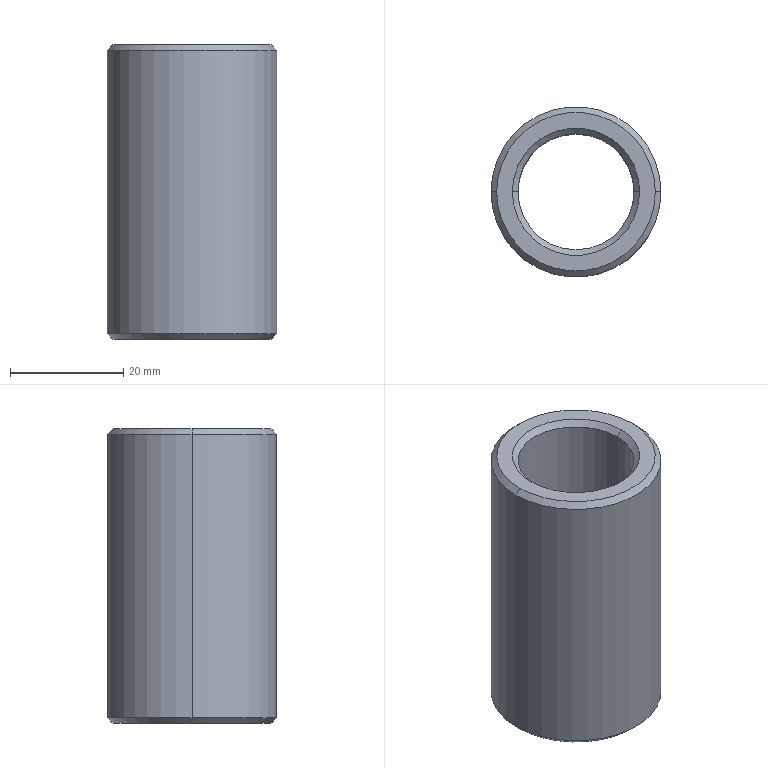Part | SolidWorks | features Chamfer 1, Extrusion 1 | 1 solid | 14 faces | box 30 x 30 x 52 mm | volume 19435 mm3 | cone 8 | cylinder 4 | plane 2 | commonest cylinder face diameters 20.5 x2 30 x2
STEP:
#1=CARTESIAN_POINT('',(-10.25,0.,25.));
#2=VERTEX_POINT('',#1);
#3=CARTESIAN_POINT('',(10.25,0.,25.));
#4=VERTEX_POINT('',#3);
#5=CARTESIAN_POINT('',(0.,0.,25.));
#6=DIRECTION('',(0.,0.,1.));
#7=DIRECTION('',(1.,0.,0.));
#8=AXIS2_PLACEMENT_3D('',#5,#6,#7);
#9=CIRCLE('',#8,10.25);
#10=EDGE_CURVE('',#2,#4,#9,.T.);
#11=ORIENTED_EDGE('',*,*,#10,.F.);
#12=CARTESIAN_POINT('',(-11.25,0.,26.));
#13=VERTEX_POINT('',#12);
#14=CARTESIAN_POINT('',(-10.25,0.,25.));
#15=DIRECTION('',(-0.7071,0.,0.7071));
#16=VECTOR('',#15,1000.);
#17=LINE('',#14,#16);
#18=EDGE_CURVE('',#2,#13,#17,.T.);
#19=ORIENTED_EDGE('',*,*,#18,.T.);
#20=CARTESIAN_POINT('',(11.25,0.,26.));
#21=VERTEX_POINT('',#20);
#22=CARTESIAN_POINT('',(0.,0.,26.));
#23=DIRECTION('',(0.,0.,-1.));
#24=DIRECTION('',(1.,0.,0.));
#25=AXIS2_PLACEMENT_3D('',#22,#23,#24);
#26=CIRCLE('',#25,11.25);
#27=EDGE_CURVE('',#21,#13,#26,.T.);
#28=ORIENTED_EDGE('',*,*,#27,.F.);
#29=CARTESIAN_POINT('',(10.25,0.,25.));
#30=DIRECTION('',(0.7071,0.,0.7071));
#31=VECTOR('',#30,1000.);
#32=LINE('',#29,#31);
#33=EDGE_CURVE('',#4,#21,#32,.T.);
#34=ORIENTED_EDGE('',*,*,#33,.F.);
#35=EDGE_LOOP('',(#11,#19,#28,#34));
#36=FACE_OUTER_BOUND('',#35,.T.);
#37=CARTESIAN_POINT('',(0.,0.,25.));
#38=DIRECTION('',(0.,0.,1.));
#39=DIRECTION('',(1.,0.,0.));
#40=AXIS2_PLACEMENT_3D('',#37,#38,#39);
#41=CONICAL_SURFACE('',#40,10.25,0.7854);
#42=ADVANCED_FACE('',(#36),#41,.F.);
#43=CARTESIAN_POINT('',(14.,0.,26.));
#44=VERTEX_POINT('',#43);
#45=CARTESIAN_POINT('',(-14.,0.,26.));
#46=VERTEX_POINT('',#45);
#47=CARTESIAN_POINT('',(0.,0.,26.));
#48=DIRECTION('',(0.,0.,1.));
#49=DIRECTION('',(1.,0.,0.));
#50=AXIS2_PLACEMENT_3D('',#47,#48,#49);
#51=CIRCLE('',#50,14.);
#52=EDGE_CURVE('',#44,#46,#51,.T.);
#53=ORIENTED_EDGE('',*,*,#52,.F.);
#54=CARTESIAN_POINT('',(15.,0.,25.));
#55=VERTEX_POINT('',#54);
#56=CARTESIAN_POINT('',(14.,0.,26.));
#57=DIRECTION('',(0.7071,0.,-0.7071));
#58=VECTOR('',#57,1000.);
#59=LINE('',#56,#58);
#60=EDGE_CURVE('',#44,#55,#59,.T.);
#61=ORIENTED_EDGE('',*,*,#60,.T.);
#62=CARTESIAN_POINT('',(-15.,0.,25.));
#63=VERTEX_POINT('',#62);
#64=CARTESIAN_POINT('',(0.,0.,25.));
#65=DIRECTION('',(0.,0.,-1.));
#66=DIRECTION('',(1.,0.,0.));
#67=AXIS2_PLACEMENT_3D('',#64,#65,#66);
#68=CIRCLE('',#67,15.);
#69=EDGE_CURVE('',#63,#55,#68,.T.);
#70=ORIENTED_EDGE('',*,*,#69,.F.);
#71=CARTESIAN_POINT('',(-14.,0.,26.));
#72=DIRECTION('',(-0.7071,0.,-0.7071));
#73=VECTOR('',#72,1000.);
#74=LINE('',#71,#73);
#75=EDGE_CURVE('',#46,#63,#74,.T.);
#76=ORIENTED_EDGE('',*,*,#75,.F.);
#77=EDGE_LOOP('',(#53,#61,#70,#76));
#78=FACE_OUTER_BOUND('',#77,.T.);
#79=CARTESIAN_POINT('',(0.,0.,26.));
#80=DIRECTION('',(0.,0.,-1.));
#81=DIRECTION('',(-1.,0.,0.));
#82=AXIS2_PLACEMENT_3D('',#79,#80,#81);
#83=CONICAL_SURFACE('',#82,14.,0.7854);
#84=ADVANCED_FACE('',(#78),#83,.T.);
#85=CARTESIAN_POINT('',(10.25,0.,-25.));
#86=VERTEX_POINT('',#85);
#87=CARTESIAN_POINT('',(-10.25,0.,-25.));
#88=VERTEX_POINT('',#87);
#89=CARTESIAN_POINT('',(0.,0.,-25.));
#90=DIRECTION('',(0.,0.,-1.));
#91=DIRECTION('',(1.,0.,0.));
#92=AXIS2_PLACEMENT_3D('',#89,#90,#91);
#93=CIRCLE('',#92,10.25);
#94=EDGE_CURVE('',#86,#88,#93,.T.);
#95=ORIENTED_EDGE('',*,*,#94,.F.);
#96=CARTESIAN_POINT('',(11.25,0.,-26.));
#97=VERTEX_POINT('',#96);
#98=CARTESIAN_POINT('',(11.25,0.,-26.));
#99=DIRECTION('',(0.7071,0.,-0.7071));
#100=VECTOR('',#99,1000.);
#101=LINE('',#98,#100);
#102=EDGE_CURVE('',#86,#97,#101,.T.);
#103=ORIENTED_EDGE('',*,*,#102,.T.);
#104=CARTESIAN_POINT('',(-11.25,0.,-26.));
#105=VERTEX_POINT('',#104);
#106=CARTESIAN_POINT('',(0.,0.,-26.));
#107=DIRECTION('',(0.,0.,1.));
#108=DIRECTION('',(1.,0.,0.));
#109=AXIS2_PLACEMENT_3D('',#106,#107,#108);
#110=CIRCLE('',#109,11.25);
#111=EDGE_CURVE('',#105,#97,#110,.T.);
#112=ORIENTED_EDGE('',*,*,#111,.F.);
#113=CARTESIAN_POINT('',(-11.25,0.,-26.));
#114=DIRECTION('',(-0.7071,0.,-0.7071));
#115=VECTOR('',#114,1000.);
#116=LINE('',#113,#115);
#117=EDGE_CURVE('',#88,#105,#116,.T.);
#118=ORIENTED_EDGE('',*,*,#117,.F.);
#119=EDGE_LOOP('',(#95,#103,#112,#118));
#120=FACE_OUTER_BOUND('',#119,.T.);
#121=CARTESIAN_POINT('',(0.,0.,-26.));
#122=DIRECTION('',(0.,0.,-1.));
#123=DIRECTION('',(-1.,0.,0.));
#124=AXIS2_PLACEMENT_3D('',#121,#122,#123);
#125=CONICAL_SURFACE('',#124,11.25,0.7854);
#126=ADVANCED_FACE('',(#120),#125,.F.);
#127=CARTESIAN_POINT('',(-14.,0.,-26.));
#128=VERTEX_POINT('',#127);
#129=CARTESIAN_POINT('',(14.,0.,-26.));
#130=VERTEX_POINT('',#129);
#131=CARTESIAN_POINT('',(0.,0.,-26.));
#132=DIRECTION('',(0.,0.,-1.));
#133=DIRECTION('',(1.,0.,0.));
#134=AXIS2_PLACEMENT_3D('',#131,#132,#133);
#135=CIRCLE('',#134,14.);
#136=EDGE_CURVE('',#128,#130,#135,.T.);
#137=ORIENTED_EDGE('',*,*,#136,.F.);
#138=CARTESIAN_POINT('',(-15.,0.,-25.));
#139=VERTEX_POINT('',#138);
#140=CARTESIAN_POINT('',(-15.,0.,-25.));
#141=DIRECTION('',(-0.7071,0.,0.7071));
#142=VECTOR('',#141,1000.);
#143=LINE('',#140,#142);
#144=EDGE_CURVE('',#128,#139,#143,.T.);
#145=ORIENTED_EDGE('',*,*,#144,.T.);
#146=CARTESIAN_POINT('',(15.,0.,-25.));
#147=VERTEX_POINT('',#146);
#148=CARTESIAN_POINT('',(0.,0.,-25.));
#149=DIRECTION('',(0.,0.,1.));
#150=DIRECTION('',(1.,0.,0.));
#151=AXIS2_PLACEMENT_3D('',#148,#149,#150);
#152=CIRCLE('',#151,15.);
#153=EDGE_CURVE('',#147,#139,#152,.T.);
#154=ORIENTED_EDGE('',*,*,#153,.F.);
#155=CARTESIAN_POINT('',(15.,0.,-25.));
#156=DIRECTION('',(0.7071,0.,0.7071));
#157=VECTOR('',#156,1000.);
#158=LINE('',#155,#157);
#159=EDGE_CURVE('',#130,#147,#158,.T.);
#160=ORIENTED_EDGE('',*,*,#159,.F.);
#161=EDGE_LOOP('',(#137,#145,#154,#160));
#162=FACE_OUTER_BOUND('',#161,.T.);
#163=CARTESIAN_POINT('',(0.,0.,-25.));
#164=DIRECTION('',(0.,0.,1.));
#165=DIRECTION('',(1.,0.,0.));
#166=AXIS2_PLACEMENT_3D('',#163,#164,#165);
#167=CONICAL_SURFACE('',#166,15.,0.7854);
#168=ADVANCED_FACE('',(#162),#167,.T.);
#169=ORIENTED_EDGE('',*,*,#10,.T.);
#170=CARTESIAN_POINT('',(10.25,0.,26.));
#171=DIRECTION('',(0.,0.,-1.));
#172=VECTOR('',#171,1000.);
#173=LINE('',#170,#172);
#174=EDGE_CURVE('',#4,#86,#173,.T.);
#175=ORIENTED_EDGE('',*,*,#174,.T.);
#176=ORIENTED_EDGE('',*,*,#94,.T.);
#177=CARTESIAN_POINT('',(-10.25,0.,26.));
#178=DIRECTION('',(0.,0.,-1.));
#179=VECTOR('',#178,1000.);
#180=LINE('',#177,#179);
#181=EDGE_CURVE('',#2,#88,#180,.T.);
#182=ORIENTED_EDGE('',*,*,#181,.F.);
#183=EDGE_LOOP('',(#169,#175,#176,#182));
#184=FACE_OUTER_BOUND('',#183,.T.);
#185=CARTESIAN_POINT('',(0.,0.,26.));
#186=DIRECTION('',(0.,0.,-1.));
#187=DIRECTION('',(-1.,0.,0.));
#188=AXIS2_PLACEMENT_3D('',#185,#186,#187);
#189=CYLINDRICAL_SURFACE('',#188,10.25);
#190=ADVANCED_FACE('',(#184),#189,.F.);
#191=ORIENTED_EDGE('',*,*,#69,.T.);
#192=CARTESIAN_POINT('',(15.,0.,26.));
#193=DIRECTION('',(0.,0.,-1.));
#194=VECTOR('',#193,1000.);
#195=LINE('',#192,#194);
#196=EDGE_CURVE('',#55,#147,#195,.T.);
#197=ORIENTED_EDGE('',*,*,#196,.T.);
#198=ORIENTED_EDGE('',*,*,#153,.T.);
#199=CARTESIAN_POINT('',(-15.,0.,26.));
#200=DIRECTION('',(0.,0.,-1.));
#201=VECTOR('',#200,1000.);
#202=LINE('',#199,#201);
#203=EDGE_CURVE('',#63,#139,#202,.T.);
#204=ORIENTED_EDGE('',*,*,#203,.F.);
#205=EDGE_LOOP('',(#191,#197,#198,#204));
#206=FACE_OUTER_BOUND('',#205,.T.);
#207=CARTESIAN_POINT('',(0.,0.,26.));
#208=DIRECTION('',(0.,0.,-1.));
#209=DIRECTION('',(-1.,0.,0.));
#210=AXIS2_PLACEMENT_3D('',#207,#208,#209);
#211=CYLINDRICAL_SURFACE('',#210,15.);
#212=ADVANCED_FACE('',(#206),#211,.T.);
#213=CARTESIAN_POINT('',(0.,0.,26.));
#214=DIRECTION('',(0.,0.,1.));
#215=DIRECTION('',(1.,0.,0.));
#216=AXIS2_PLACEMENT_3D('',#213,#214,#215);
#217=CIRCLE('',#216,14.);
#218=EDGE_CURVE('',#46,#44,#217,.T.);
#219=ORIENTED_EDGE('',*,*,#218,.T.);
#220=ORIENTED_EDGE('',*,*,#52,.T.);
#221=EDGE_LOOP('',(#219,#220));
#222=FACE_OUTER_BOUND('',#221,.T.);
#223=ORIENTED_EDGE('',*,*,#27,.T.);
#224=CARTESIAN_POINT('',(0.,0.,26.));
#225=DIRECTION('',(0.,0.,-1.));
#226=DIRECTION('',(1.,0.,0.));
#227=AXIS2_PLACEMENT_3D('',#224,#225,#226);
#228=CIRCLE('',#227,11.25);
#229=EDGE_CURVE('',#13,#21,#228,.T.);
#230=ORIENTED_EDGE('',*,*,#229,.T.);
#231=EDGE_LOOP('',(#223,#230));
#232=FACE_BOUND('',#231,.T.);
#233=CARTESIAN_POINT('',(0.,0.,26.));
#234=DIRECTION('',(0.,0.,1.));
#235=DIRECTION('',(1.,0.,0.));
#236=AXIS2_PLACEMENT_3D('',#233,#234,#235);
#237=PLANE('',#236);
#238=ADVANCED_FACE('',(#222,#232),#237,.T.);
#239=CARTESIAN_POINT('',(0.,0.,-26.));
#240=DIRECTION('',(0.,0.,-1.));
#241=DIRECTION('',(1.,0.,0.));
#242=AXIS2_PLACEMENT_3D('',#239,#240,#241);
#243=CIRCLE('',#242,14.);
#244=EDGE_CURVE('',#130,#128,#243,.T.);
#245=ORIENTED_EDGE('',*,*,#244,.T.);
#246=ORIENTED_EDGE('',*,*,#136,.T.);
#247=EDGE_LOOP('',(#245,#246));
#248=FACE_OUTER_BOUND('',#247,.T.);
#249=ORIENTED_EDGE('',*,*,#111,.T.);
#250=CARTESIAN_POINT('',(0.,0.,-26.));
#251=DIRECTION('',(0.,0.,1.));
#252=DIRECTION('',(1.,0.,0.));
#253=AXIS2_PLACEMENT_3D('',#250,#251,#252);
#254=CIRCLE('',#253,11.25);
#255=EDGE_CURVE('',#97,#105,#254,.T.);
#256=ORIENTED_EDGE('',*,*,#255,.T.);
#257=EDGE_LOOP('',(#249,#256));
#258=FACE_BOUND('',#257,.T.);
#259=CARTESIAN_POINT('',(0.,0.,-26.));
#260=DIRECTION('',(0.,0.,1.));
#261=DIRECTION('',(1.,0.,0.));
#262=AXIS2_PLACEMENT_3D('',#259,#260,#261);
#263=PLANE('',#262);
#264=ADVANCED_FACE('',(#248,#258),#263,.F.);
#265=ORIENTED_EDGE('',*,*,#196,.F.);
#266=CARTESIAN_POINT('',(0.,0.,25.));
#267=DIRECTION('',(0.,0.,-1.));
#268=DIRECTION('',(1.,0.,0.));
#269=AXIS2_PLACEMENT_3D('',#266,#267,#268);
#270=CIRCLE('',#269,15.);
#271=EDGE_CURVE('',#55,#63,#270,.T.);
#272=ORIENTED_EDGE('',*,*,#271,.T.);
#273=ORIENTED_EDGE('',*,*,#203,.T.);
#274=CARTESIAN_POINT('',(0.,0.,-25.));
#275=DIRECTION('',(0.,0.,1.));
#276=DIRECTION('',(1.,0.,0.));
#277=AXIS2_PLACEMENT_3D('',#274,#275,#276);
#278=CIRCLE('',#277,15.);
#279=EDGE_CURVE('',#139,#147,#278,.T.);
#280=ORIENTED_EDGE('',*,*,#279,.T.);
#281=EDGE_LOOP('',(#265,#272,#273,#280));
#282=FACE_OUTER_BOUND('',#281,.T.);
#283=CARTESIAN_POINT('',(0.,0.,26.));
#284=DIRECTION('',(0.,0.,-1.));
#285=DIRECTION('',(-1.,0.,0.));
#286=AXIS2_PLACEMENT_3D('',#283,#284,#285);
#287=CYLINDRICAL_SURFACE('',#286,15.);
#288=ADVANCED_FACE('',(#282),#287,.T.);
#289=ORIENTED_EDGE('',*,*,#174,.F.);
#290=CARTESIAN_POINT('',(0.,0.,25.));
#291=DIRECTION('',(0.,0.,1.));
#292=DIRECTION('',(1.,0.,0.));
#293=AXIS2_PLACEMENT_3D('',#290,#291,#292);
#294=CIRCLE('',#293,10.25);
#295=EDGE_CURVE('',#4,#2,#294,.T.);
#296=ORIENTED_EDGE('',*,*,#295,.T.);
#297=ORIENTED_EDGE('',*,*,#181,.T.);
#298=CARTESIAN_POINT('',(0.,0.,-25.));
#299=DIRECTION('',(0.,0.,-1.));
#300=DIRECTION('',(1.,0.,0.));
#301=AXIS2_PLACEMENT_3D('',#298,#299,#300);
#302=CIRCLE('',#301,10.25);
#303=EDGE_CURVE('',#88,#86,#302,.T.);
#304=ORIENTED_EDGE('',*,*,#303,.T.);
#305=EDGE_LOOP('',(#289,#296,#297,#304));
#306=FACE_OUTER_BOUND('',#305,.T.);
#307=CARTESIAN_POINT('',(0.,0.,26.));
#308=DIRECTION('',(0.,0.,-1.));
#309=DIRECTION('',(-1.,0.,0.));
#310=AXIS2_PLACEMENT_3D('',#307,#308,#309);
#311=CYLINDRICAL_SURFACE('',#310,10.25);
#312=ADVANCED_FACE('',(#306),#311,.F.);
#313=ORIENTED_EDGE('',*,*,#144,.F.);
#314=ORIENTED_EDGE('',*,*,#244,.F.);
#315=ORIENTED_EDGE('',*,*,#159,.T.);
#316=ORIENTED_EDGE('',*,*,#279,.F.);
#317=EDGE_LOOP('',(#313,#314,#315,#316));
#318=FACE_OUTER_BOUND('',#317,.T.);
#319=CARTESIAN_POINT('',(0.,0.,-25.));
#320=DIRECTION('',(0.,0.,1.));
#321=DIRECTION('',(1.,0.,0.));
#322=AXIS2_PLACEMENT_3D('',#319,#320,#321);
#323=CONICAL_SURFACE('',#322,15.,0.7854);
#324=ADVANCED_FACE('',(#318),#323,.T.);
#325=ORIENTED_EDGE('',*,*,#102,.F.);
#326=ORIENTED_EDGE('',*,*,#303,.F.);
#327=ORIENTED_EDGE('',*,*,#117,.T.);
#328=ORIENTED_EDGE('',*,*,#255,.F.);
#329=EDGE_LOOP('',(#325,#326,#327,#328));
#330=FACE_OUTER_BOUND('',#329,.T.);
#331=CARTESIAN_POINT('',(0.,0.,-26.));
#332=DIRECTION('',(0.,0.,-1.));
#333=DIRECTION('',(-1.,0.,0.));
#334=AXIS2_PLACEMENT_3D('',#331,#332,#333);
#335=CONICAL_SURFACE('',#334,11.25,0.7854);
#336=ADVANCED_FACE('',(#330),#335,.F.);
#337=ORIENTED_EDGE('',*,*,#60,.F.);
#338=ORIENTED_EDGE('',*,*,#218,.F.);
#339=ORIENTED_EDGE('',*,*,#75,.T.);
#340=ORIENTED_EDGE('',*,*,#271,.F.);
#341=EDGE_LOOP('',(#337,#338,#339,#340));
#342=FACE_OUTER_BOUND('',#341,.T.);
#343=CARTESIAN_POINT('',(0.,0.,26.));
#344=DIRECTION('',(0.,0.,-1.));
#345=DIRECTION('',(-1.,0.,0.));
#346=AXIS2_PLACEMENT_3D('',#343,#344,#345);
#347=CONICAL_SURFACE('',#346,14.,0.7854);
#348=ADVANCED_FACE('',(#342),#347,.T.);
#349=ORIENTED_EDGE('',*,*,#18,.F.);
#350=ORIENTED_EDGE('',*,*,#295,.F.);
#351=ORIENTED_EDGE('',*,*,#33,.T.);
#352=ORIENTED_EDGE('',*,*,#229,.F.);
#353=EDGE_LOOP('',(#349,#350,#351,#352));
#354=FACE_OUTER_BOUND('',#353,.T.);
#355=CARTESIAN_POINT('',(0.,0.,25.));
#356=DIRECTION('',(0.,0.,1.));
#357=DIRECTION('',(1.,0.,0.));
#358=AXIS2_PLACEMENT_3D('',#355,#356,#357);
#359=CONICAL_SURFACE('',#358,10.25,0.7854);
#360=ADVANCED_FACE('',(#354),#359,.F.);
#361=CLOSED_SHELL('',(#42,#84,#126,#168,#190,#212,#238,#264,#288,#312,#324,#336,#348,#360));
#362=MANIFOLD_SOLID_BREP('',#361);
#363=CARTESIAN_POINT('',(0.,0.,0.));
#364=DIRECTION('',(0.,0.,1.));
#365=DIRECTION('',(1.,0.,0.));
#366=AXIS2_PLACEMENT_3D('',#363,#364,#365);
#367=(LENGTH_UNIT()NAMED_UNIT(*)SI_UNIT(.MILLI.,.METRE.));
#368=UNCERTAINTY_MEASURE_WITH_UNIT(LENGTH_MEASURE(0.00001),#367,'','');
#369=(NAMED_UNIT(*)PLANE_ANGLE_UNIT()SI_UNIT($,.RADIAN.));
#370=(NAMED_UNIT(*)SI_UNIT($,.STERADIAN.)SOLID_ANGLE_UNIT());
#371=(GEOMETRIC_REPRESENTATION_CONTEXT(3)GLOBAL_UNCERTAINTY_ASSIGNED_CONTEXT((#368))GLOBAL_UNIT_ASSIGNED_CONTEXT((#367,#369,#370))REPRESENTATION_CONTEXT('',''));
#372=ADVANCED_BREP_SHAPE_REPRESENTATION('',(#362,#366),#371);